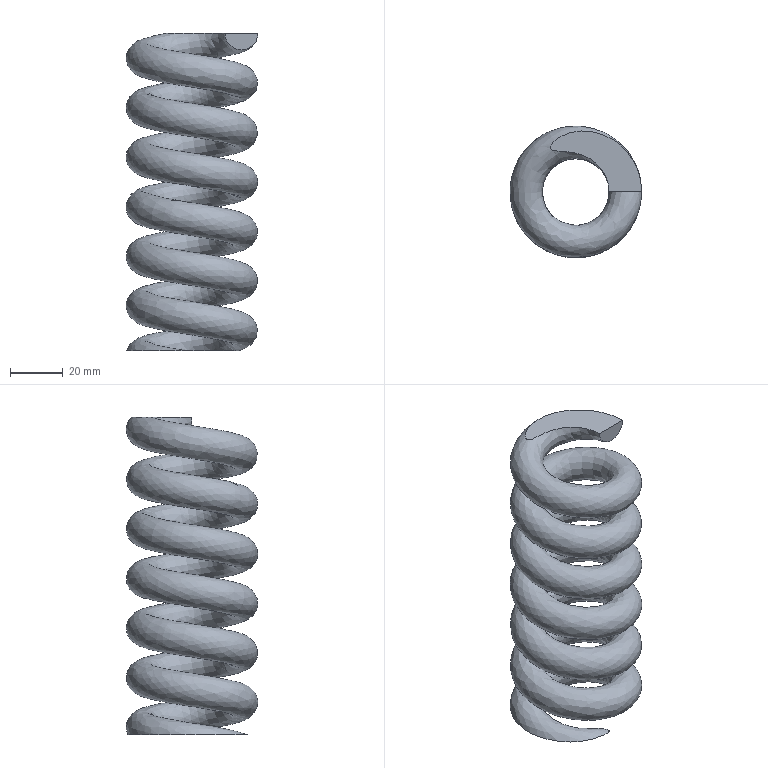Part | NX | features solid 2 | 1 solid | 4 faces | volume 89697 mm3 | plane 3 | spline 1